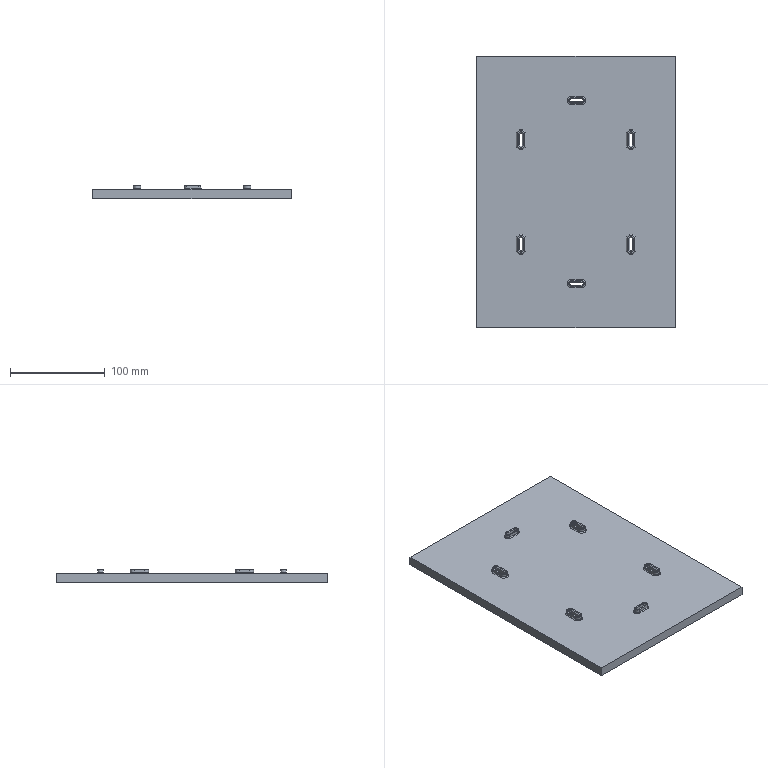Part | NX | features BREP 1 | 1 solid | 108 faces | box 209.8 x 286.897 x 14 mm | volume 601410 mm3 | plane 52 | cylinder 32 | cone 16 | torus 8 | commonest cylinder face diameters 3.173 x8 8.173 x8 2 x4 3.207 x4 6.207 x4 0.8 x2